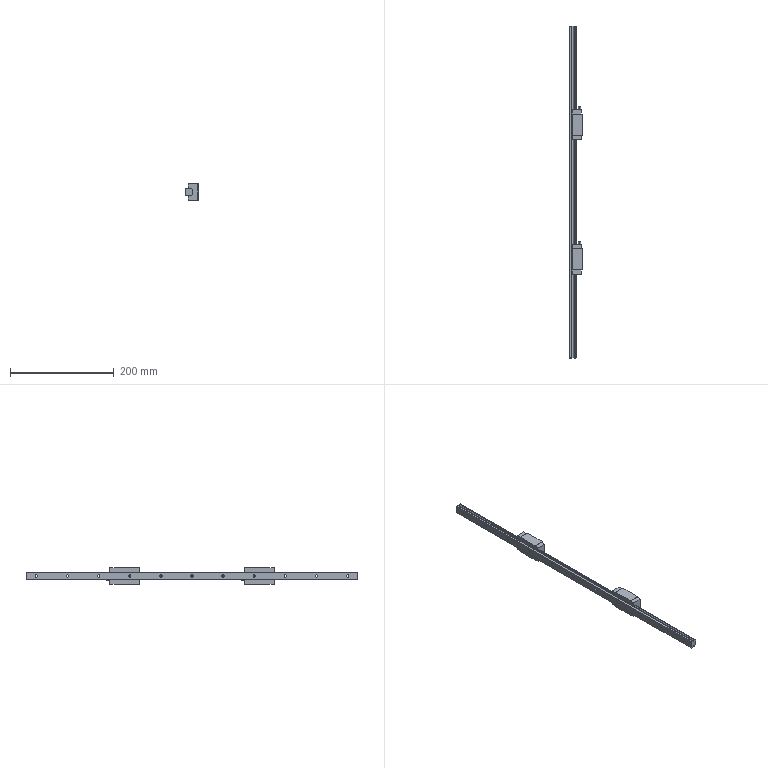Part | NX | features BREP 3 | 3 solids | 171 faces | box 24 x 640 x 34 mm | volume 168254 mm3 | plane 83 | cylinder 68 | cone 16 | torus 4 | commonest cylinder face diameters 4.5 x30 7.5 x22 3.3 x16